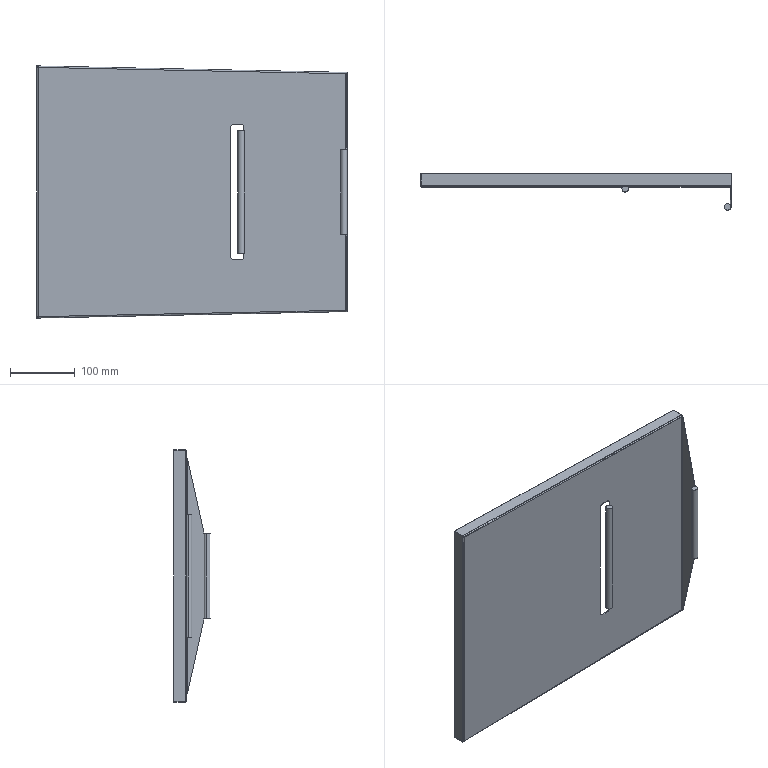Part | SolidWorks | features ICE 4, EdgeFlange 2, CornerFeat 1, Fillet 1, FlatPattern 1, SMBaseFlange 1, SheetMetal 1 | 3 solids | 64 faces | box 480 x 56.239 x 389.95 mm | volume 276290 mm3 | plane 42 | cylinder 18 | spline 4 | commonest cylinder face diameters 10 x8 4.4 x6 2 x4